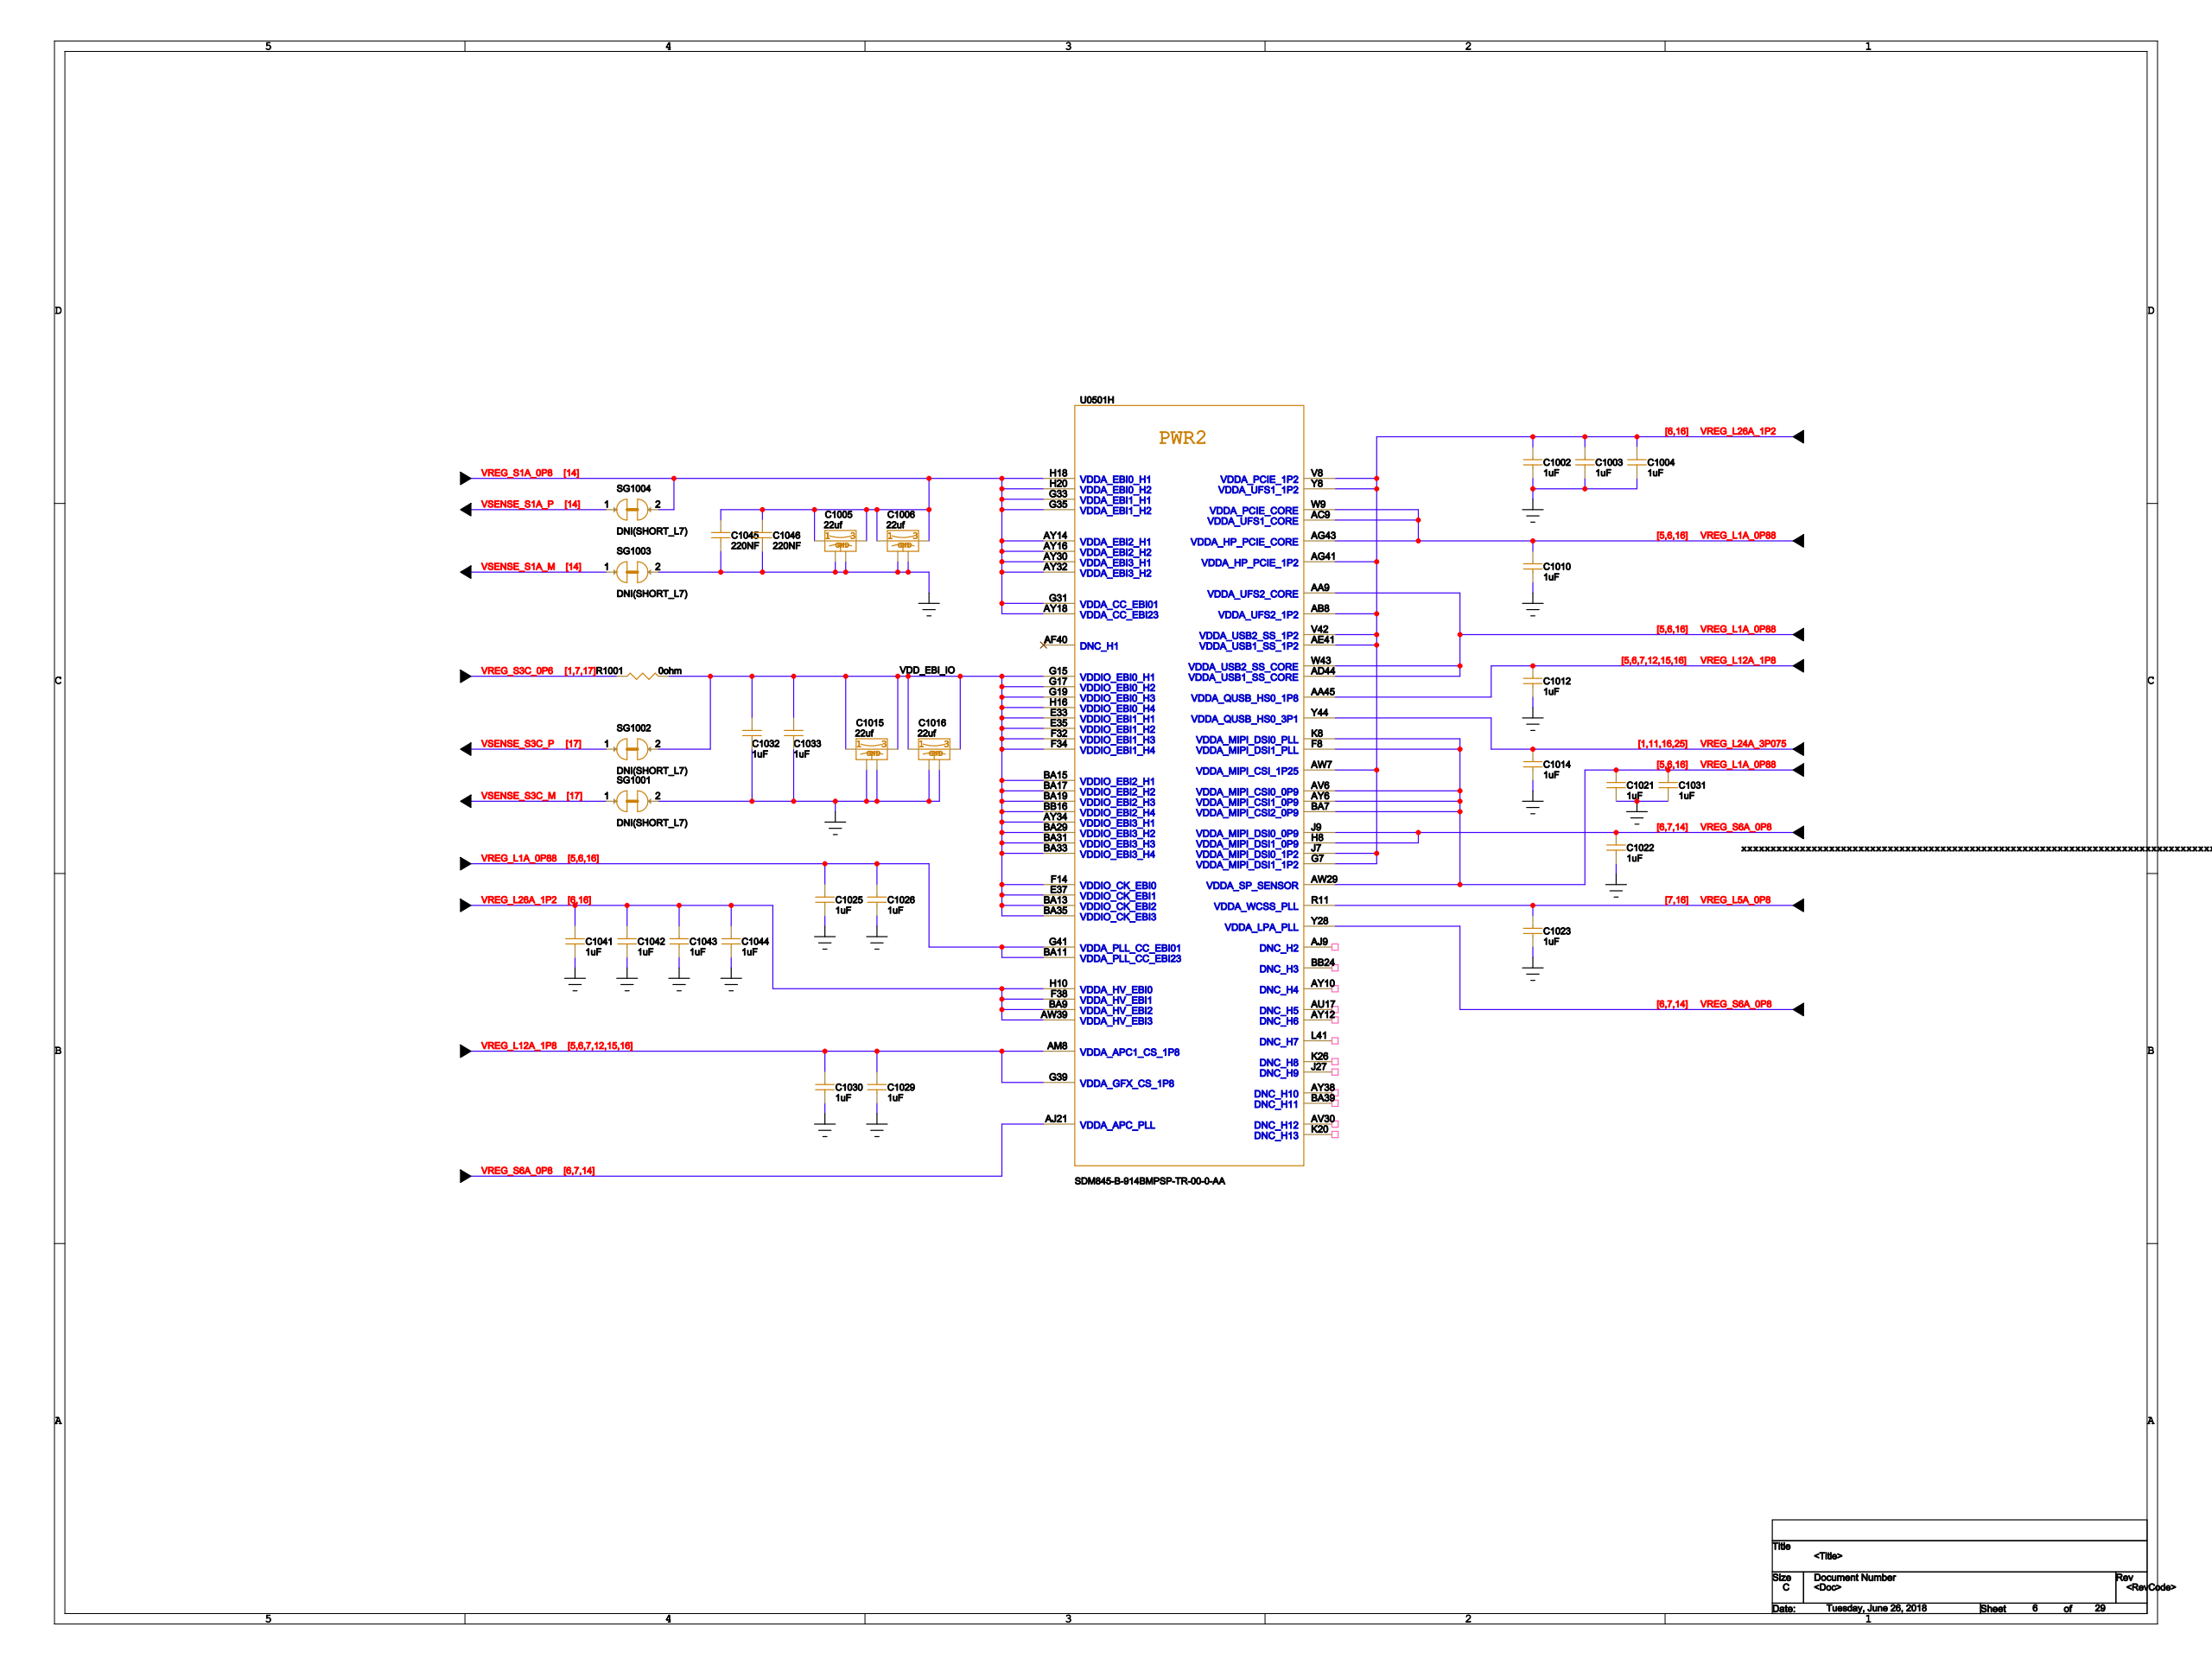Circuit board | Cadence Allegro | 802 parts | 566 nets | one sheet of the schematic
Parts on this sheet (reference | value | footprint):
C1002 | 1uF | C0201
C1003 | 1uF | C0201
C1004 | 1uF | C0201
C1005 | 22uf | NFMJMPC226R0G3
C1006 | 22uf | NFMJMPC226R0G3
C1010 | 1uF | C0201
C1012 | 1uF | C0201
C1014 | 1uF | C0201
C1015 | 22uf | NFMJMPC226R0G3
C1016 | 22uf | NFMJMPC226R0G3
C1021 | 1uF | C0201
C1022 | 1uF | C0201
C1023 | 1uF | C0201
C1025 | 1uF | C0201
C1026 | 1uF | C0201
C1029 | 1uF | C0201
C1030 | 1uF | C0201
C1031 | 1uF | C0201
C1032 | 1uF | C0201
C1033 | 1uF | C0201
C1041 | 1uF | C0201
C1042 | 1uF | C0201
C1043 | 1uF | C0201
C1044 | 1uF | C0201
C1045 | 220NF | C0201
C1046 | 220NF | C0201
R1001 | 0OHM | R0201
SG1001 | DNI(SHORT_L7) | SHORT_L7_2REC08X12
SG1002 | DNI(SHORT_L7) | SHORT_L7_2REC08X12
SG1003 | DNI(SHORT_L7) | SHORT_L7_2REC08X12
SG1004 | DNI(SHORT_L7) | SHORT_L7_2REC08X12
U0501 | SDM845-B-914BMPSP-TR-00-0-AA | BGA914_12P4X12P4_0P58_0P35
Nets of these parts (net: part-pin ...):
GND: C1002-2 C1003-2 C1004-2 C1005-2 C1005-4 C1006-2 C1006-4 C1010-2 C1012-2 C1014-2 C1015-2 C1015-4 C1016-2 C1016-4 C1021-2 C1022-2 C1023-2 C1025-2 C1026-2 C1029-2 C1030-2 C1031-2 C1032-2 C1033-2 C1041-2 C1042-2 C1043-2 C1044-2 C1045-2 C1046-2 SG1001-2 SG1003-2
VREG_L24A_3P075: C1014-1 U0501-Y44
VREG_S3C_0P6: R1001-1
VREG_S6A_0P8: C1022-1 U0501-AJ21 U0501-H8 U0501-J9 U0501-Y28
VDD_EBI_IO: C1015-1 C1015-3 C1016-1 C1016-3 C1032-1 C1033-1 R1001-2 SG1002-2 U0501-AY34 U0501-BA13 U0501-BA15 U0501-BA17 U0501-BA19 U0501-BA29 U0501-BA31 U0501-BA33 U0501-BA35 U0501-BB16 U0501-E33 U0501-E35 U0501-E37 U0501-F14 U0501-F32 U0501-F34 U0501-G15 U0501-G17 U0501-G19 U0501-H16
VREG_L1A_0P88: C1010-1 C1021-1 C1025-1 C1026-1 C1031-1 U0501-AA9 U0501-AC9 U0501-AD44 U0501-AG43 U0501-AV6 U0501-AW29 U0501-AY6 U0501-BA7 U0501-BA11 U0501-F8 U0501-G41 U0501-K8 U0501-W9 U0501-W43
VREG_L12A_1P8: C1012-1 C1029-1 C1030-1 U0501-AA45 U0501-AM8 U0501-G39
VREG_L26A_1P2: C1002-1 C1003-1 C1004-1 C1041-1 C1042-1 C1043-1 C1044-1 U0501-AB8 U0501-AE41 U0501-AG41 U0501-AW7 U0501-AW39 U0501-BA9 U0501-F38 U0501-G7 U0501-H10 U0501-J7 U0501-V8 U0501-V42 U0501-Y8
VREG_L5A_0P8: C1023-1 U0501-R11
VREG_S1A_0P8: C1005-1 C1005-3 C1006-1 C1006-3 C1045-1 C1046-1 SG1004-2 U0501-AY14 U0501-AY16 U0501-AY18 U0501-AY30 U0501-AY32 U0501-G31 U0501-G33 U0501-G35 U0501-H18 U0501-H20
VSENSE_S3C_M: SG1001-1
VSENSE_S3C_P: SG1002-1
VSENSE_S1A_M: SG1003-1
VSENSE_S1A_P: SG1004-1